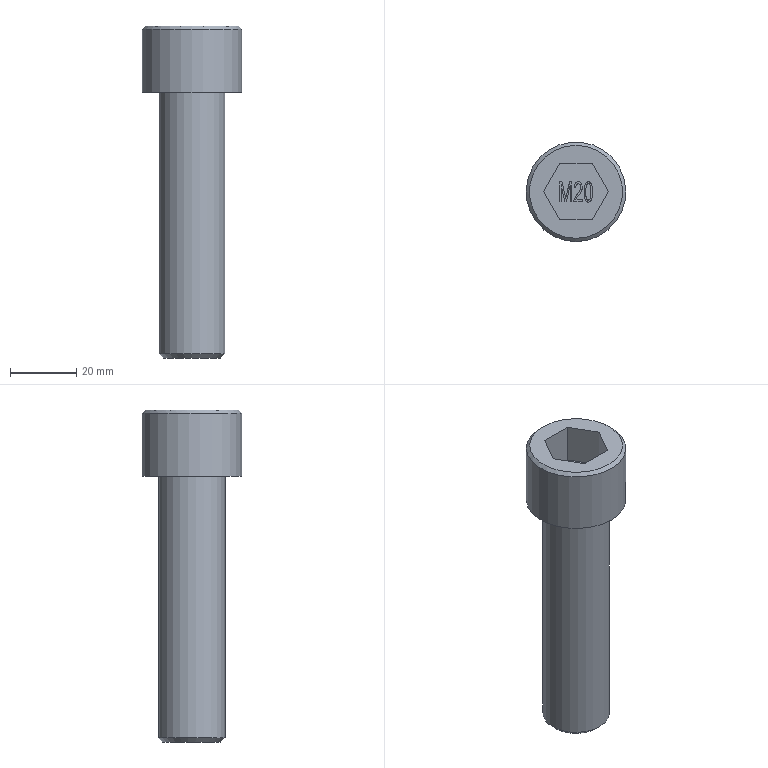Part | STEP file | M20-1 | 1 solid | 41 faces | box 30 x 30 x 100 mm | volume 36177 mm3 | plane 29 | other 8 | cylinder 2 | cone 2 | commonest cylinder face diameters 20 x1 30 x1